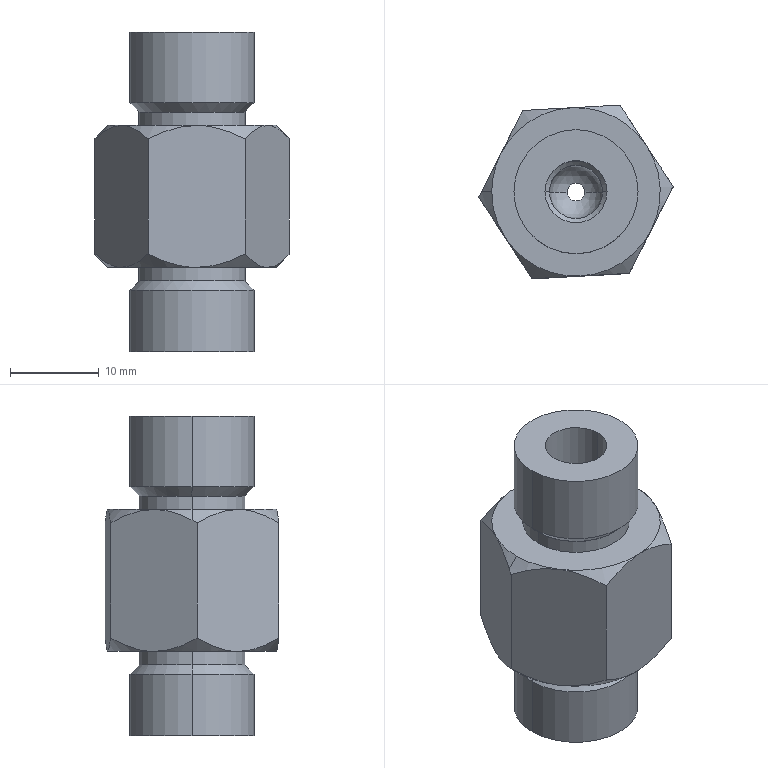Part | SolidWorks | features ICE 4, RevCut 2, StudWizard 2, Extrusion 1 | 1 solid | 64 faces | box 21.906 x 19.575 x 36 mm | volume 6912 mm3 | plane 24 | cone 22 | cylinder 16 | sphere 2 | commonest cylinder face diameters 12 x4 14 x4 2 x2 5 x2 6 x2 7 x2